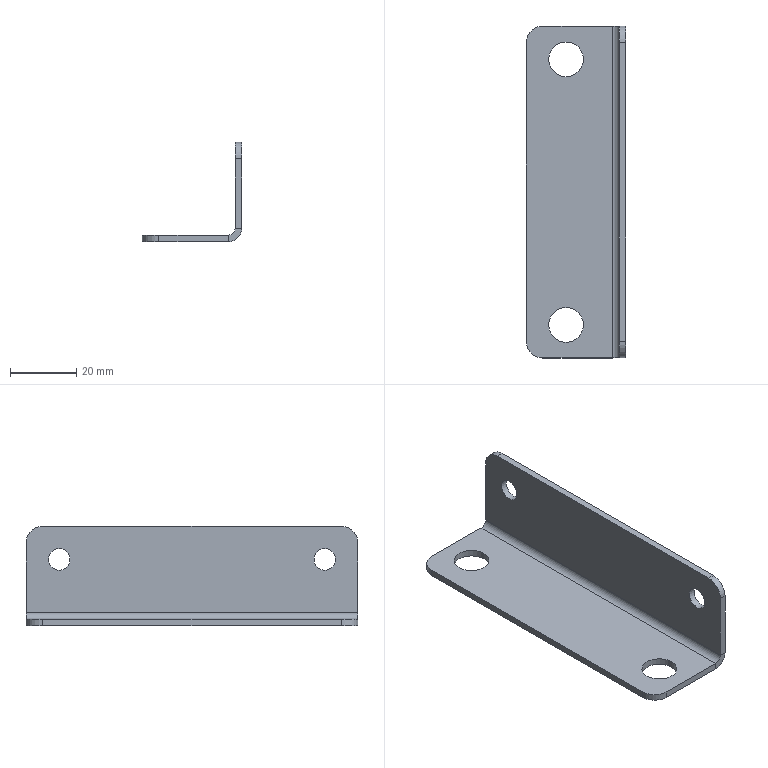Part | STEP file | JBJ-P-1006-07 | 1 solid | 22 faces | box 30 x 100 x 30 mm | volume 10820 mm3 | plane 12 | cylinder 10 | commonest cylinder face diameters 10 x4 6.5 x2 10.5 x2 4 x1 8 x1
STEP:
#1=CARTESIAN_POINT('',(30.,100.,4.));
#2=VERTEX_POINT('',#1);
#3=CARTESIAN_POINT('',(28.,100.,4.));
#4=VERTEX_POINT('',#3);
#5=CARTESIAN_POINT('',(30.,100.,4.));
#6=DIRECTION('',(-1.,0.,0.));
#7=VECTOR('',#6,1000.);
#8=LINE('',#5,#7);
#9=EDGE_CURVE('',#2,#4,#8,.T.);
#10=ORIENTED_EDGE('',*,*,#9,.F.);
#11=CARTESIAN_POINT('',(26.,100.,0.));
#12=VERTEX_POINT('',#11);
#13=CARTESIAN_POINT('',(26.,100.,4.));
#14=DIRECTION('',(0.,-1.,0.));
#15=DIRECTION('',(0.,0.,1.));
#16=AXIS2_PLACEMENT_3D('',#13,#14,#15);
#17=CIRCLE('',#16,4.);
#18=EDGE_CURVE('',#12,#2,#17,.T.);
#19=ORIENTED_EDGE('',*,*,#18,.F.);
#20=CARTESIAN_POINT('',(26.,100.,2.));
#21=VERTEX_POINT('',#20);
#22=CARTESIAN_POINT('',(26.,100.,2.));
#23=DIRECTION('',(0.,0.,-1.));
#24=VECTOR('',#23,1000.);
#25=LINE('',#22,#24);
#26=EDGE_CURVE('',#21,#12,#25,.T.);
#27=ORIENTED_EDGE('',*,*,#26,.F.);
#28=CARTESIAN_POINT('',(26.,100.,4.));
#29=DIRECTION('',(0.,-1.,0.));
#30=DIRECTION('',(1.,0.,0.));
#31=AXIS2_PLACEMENT_3D('',#28,#29,#30);
#32=CIRCLE('',#31,2.);
#33=EDGE_CURVE('',#21,#4,#32,.T.);
#34=ORIENTED_EDGE('',*,*,#33,.T.);
#35=EDGE_LOOP('',(#10,#19,#27,#34));
#36=FACE_OUTER_BOUND('',#35,.T.);
#37=CARTESIAN_POINT('',(30.,100.,4.));
#38=DIRECTION('',(0.,1.,0.));
#39=DIRECTION('',(0.,0.,1.));
#40=AXIS2_PLACEMENT_3D('',#37,#38,#39);
#41=PLANE('',#40);
#42=ADVANCED_FACE('',(#36),#41,.T.);
#43=CARTESIAN_POINT('',(28.,100.,25.));
#44=VERTEX_POINT('',#43);
#45=CARTESIAN_POINT('',(28.,100.,0.));
#46=DIRECTION('',(0.,0.,1.));
#47=VECTOR('',#46,1000.);
#48=LINE('',#45,#47);
#49=EDGE_CURVE('',#4,#44,#48,.T.);
#50=ORIENTED_EDGE('',*,*,#49,.T.);
#51=CARTESIAN_POINT('',(30.,100.,25.));
#52=VERTEX_POINT('',#51);
#53=CARTESIAN_POINT('',(26.,100.,25.));
#54=DIRECTION('',(1.,0.,0.));
#55=VECTOR('',#54,1000.);
#56=LINE('',#53,#55);
#57=EDGE_CURVE('',#44,#52,#56,.T.);
#58=ORIENTED_EDGE('',*,*,#57,.T.);
#59=CARTESIAN_POINT('',(30.,100.,0.));
#60=DIRECTION('',(0.,0.,1.));
#61=VECTOR('',#60,1000.);
#62=LINE('',#59,#61);
#63=EDGE_CURVE('',#2,#52,#62,.T.);
#64=ORIENTED_EDGE('',*,*,#63,.F.);
#65=ORIENTED_EDGE('',*,*,#9,.T.);
#66=EDGE_LOOP('',(#50,#58,#64,#65));
#67=FACE_OUTER_BOUND('',#66,.T.);
#68=CARTESIAN_POINT('',(26.,100.,2.));
#69=DIRECTION('',(0.,1.,0.));
#70=DIRECTION('',(0.,0.,1.));
#71=AXIS2_PLACEMENT_3D('',#68,#69,#70);
#72=PLANE('',#71);
#73=ADVANCED_FACE('',(#67),#72,.T.);
#74=CARTESIAN_POINT('',(26.,0.,0.));
#75=VERTEX_POINT('',#74);
#76=CARTESIAN_POINT('',(26.,0.,2.));
#77=VERTEX_POINT('',#76);
#78=CARTESIAN_POINT('',(26.,0.,0.));
#79=DIRECTION('',(0.,0.,1.));
#80=VECTOR('',#79,1000.);
#81=LINE('',#78,#80);
#82=EDGE_CURVE('',#75,#77,#81,.T.);
#83=ORIENTED_EDGE('',*,*,#82,.F.);
#84=CARTESIAN_POINT('',(30.,0.,4.));
#85=VERTEX_POINT('',#84);
#86=CARTESIAN_POINT('',(26.,0.,4.));
#87=DIRECTION('',(0.,-1.,0.));
#88=DIRECTION('',(0.,0.,1.));
#89=AXIS2_PLACEMENT_3D('',#86,#87,#88);
#90=CIRCLE('',#89,4.);
#91=EDGE_CURVE('',#75,#85,#90,.T.);
#92=ORIENTED_EDGE('',*,*,#91,.T.);
#93=CARTESIAN_POINT('',(28.,0.,4.));
#94=VERTEX_POINT('',#93);
#95=CARTESIAN_POINT('',(28.,0.,4.));
#96=DIRECTION('',(1.,0.,0.));
#97=VECTOR('',#96,1000.);
#98=LINE('',#95,#97);
#99=EDGE_CURVE('',#94,#85,#98,.T.);
#100=ORIENTED_EDGE('',*,*,#99,.F.);
#101=CARTESIAN_POINT('',(26.,0.,4.));
#102=DIRECTION('',(0.,-1.,0.));
#103=DIRECTION('',(1.,0.,0.));
#104=AXIS2_PLACEMENT_3D('',#101,#102,#103);
#105=CIRCLE('',#104,2.);
#106=EDGE_CURVE('',#77,#94,#105,.T.);
#107=ORIENTED_EDGE('',*,*,#106,.F.);
#108=EDGE_LOOP('',(#83,#92,#100,#107));
#109=FACE_OUTER_BOUND('',#108,.T.);
#110=CARTESIAN_POINT('',(26.,0.,0.));
#111=DIRECTION('',(0.,-1.,0.));
#112=DIRECTION('',(0.,0.,-1.));
#113=AXIS2_PLACEMENT_3D('',#110,#111,#112);
#114=PLANE('',#113);
#115=ADVANCED_FACE('',(#109),#114,.T.);
#116=CARTESIAN_POINT('',(5.,0.,2.));
#117=VERTEX_POINT('',#116);
#118=CARTESIAN_POINT('',(0.,0.,2.));
#119=DIRECTION('',(1.,0.,0.));
#120=VECTOR('',#119,1000.);
#121=LINE('',#118,#120);
#122=EDGE_CURVE('',#117,#77,#121,.T.);
#123=ORIENTED_EDGE('',*,*,#122,.F.);
#124=CARTESIAN_POINT('',(5.,0.,0.));
#125=VERTEX_POINT('',#124);
#126=CARTESIAN_POINT('',(5.,0.,4.));
#127=DIRECTION('',(0.,0.,-1.));
#128=VECTOR('',#127,1000.);
#129=LINE('',#126,#128);
#130=EDGE_CURVE('',#117,#125,#129,.T.);
#131=ORIENTED_EDGE('',*,*,#130,.T.);
#132=CARTESIAN_POINT('',(0.,0.,0.));
#133=DIRECTION('',(1.,0.,0.));
#134=VECTOR('',#133,1000.);
#135=LINE('',#132,#134);
#136=EDGE_CURVE('',#125,#75,#135,.T.);
#137=ORIENTED_EDGE('',*,*,#136,.T.);
#138=ORIENTED_EDGE('',*,*,#82,.T.);
#139=EDGE_LOOP('',(#123,#131,#137,#138));
#140=FACE_OUTER_BOUND('',#139,.T.);
#141=CARTESIAN_POINT('',(28.,0.,4.));
#142=DIRECTION('',(0.,-1.,0.));
#143=DIRECTION('',(0.,0.,-1.));
#144=AXIS2_PLACEMENT_3D('',#141,#142,#143);
#145=PLANE('',#144);
#146=ADVANCED_FACE('',(#140),#145,.T.);
#147=CARTESIAN_POINT('',(28.,90.,16.75));
#148=VERTEX_POINT('',#147);
#149=CARTESIAN_POINT('',(28.,90.,20.));
#150=DIRECTION('',(1.,0.,0.));
#151=DIRECTION('',(0.,0.,-1.));
#152=AXIS2_PLACEMENT_3D('',#149,#150,#151);
#153=CIRCLE('',#152,3.25);
#154=EDGE_CURVE('',#148,#148,#153,.T.);
#155=ORIENTED_EDGE('',*,*,#154,.T.);
#156=EDGE_LOOP('',(#155));
#157=FACE_BOUND('',#156,.T.);
#158=CARTESIAN_POINT('',(28.,10.,16.75));
#159=VERTEX_POINT('',#158);
#160=CARTESIAN_POINT('',(28.,10.,20.));
#161=DIRECTION('',(1.,0.,0.));
#162=DIRECTION('',(0.,0.,-1.));
#163=AXIS2_PLACEMENT_3D('',#160,#161,#162);
#164=CIRCLE('',#163,3.25);
#165=EDGE_CURVE('',#159,#159,#164,.T.);
#166=ORIENTED_EDGE('',*,*,#165,.T.);
#167=EDGE_LOOP('',(#166));
#168=FACE_BOUND('',#167,.T.);
#169=CARTESIAN_POINT('',(28.,95.,30.));
#170=VERTEX_POINT('',#169);
#171=CARTESIAN_POINT('',(28.,5.,30.));
#172=VERTEX_POINT('',#171);
#173=CARTESIAN_POINT('',(28.,100.,30.));
#174=DIRECTION('',(0.,-1.,0.));
#175=VECTOR('',#174,1000.);
#176=LINE('',#173,#175);
#177=EDGE_CURVE('',#170,#172,#176,.T.);
#178=ORIENTED_EDGE('',*,*,#177,.F.);
#179=CARTESIAN_POINT('',(28.,95.,25.));
#180=DIRECTION('',(-1.,0.,0.));
#181=DIRECTION('',(0.,0.,-1.));
#182=AXIS2_PLACEMENT_3D('',#179,#180,#181);
#183=CIRCLE('',#182,5.);
#184=EDGE_CURVE('',#170,#44,#183,.T.);
#185=ORIENTED_EDGE('',*,*,#184,.T.);
#186=ORIENTED_EDGE('',*,*,#49,.F.);
#187=CARTESIAN_POINT('',(28.,100.,4.));
#188=DIRECTION('',(0.,-1.,0.));
#189=VECTOR('',#188,1000.);
#190=LINE('',#187,#189);
#191=EDGE_CURVE('',#4,#94,#190,.T.);
#192=ORIENTED_EDGE('',*,*,#191,.T.);
#193=CARTESIAN_POINT('',(28.,0.,25.));
#194=VERTEX_POINT('',#193);
#195=CARTESIAN_POINT('',(28.,0.,0.));
#196=DIRECTION('',(0.,0.,1.));
#197=VECTOR('',#196,1000.);
#198=LINE('',#195,#197);
#199=EDGE_CURVE('',#94,#194,#198,.T.);
#200=ORIENTED_EDGE('',*,*,#199,.T.);
#201=CARTESIAN_POINT('',(28.,5.,25.));
#202=DIRECTION('',(-1.,0.,0.));
#203=DIRECTION('',(0.,0.,-1.));
#204=AXIS2_PLACEMENT_3D('',#201,#202,#203);
#205=CIRCLE('',#204,5.);
#206=EDGE_CURVE('',#194,#172,#205,.T.);
#207=ORIENTED_EDGE('',*,*,#206,.T.);
#208=EDGE_LOOP('',(#178,#185,#186,#192,#200,#207));
#209=FACE_OUTER_BOUND('',#208,.T.);
#210=CARTESIAN_POINT('',(28.,100.,0.));
#211=DIRECTION('',(1.,0.,0.));
#212=DIRECTION('',(0.,0.,-1.));
#213=AXIS2_PLACEMENT_3D('',#210,#211,#212);
#214=PLANE('',#213);
#215=ADVANCED_FACE('',(#157,#168,#209),#214,.F.);
#216=CARTESIAN_POINT('',(30.,95.,30.));
#217=VERTEX_POINT('',#216);
#218=CARTESIAN_POINT('',(30.,5.,30.));
#219=VERTEX_POINT('',#218);
#220=CARTESIAN_POINT('',(30.,100.,30.));
#221=DIRECTION('',(0.,-1.,0.));
#222=VECTOR('',#221,1000.);
#223=LINE('',#220,#222);
#224=EDGE_CURVE('',#217,#219,#223,.T.);
#225=ORIENTED_EDGE('',*,*,#224,.F.);
#226=CARTESIAN_POINT('',(30.,95.,30.));
#227=DIRECTION('',(-1.,0.,0.));
#228=VECTOR('',#227,1000.);
#229=LINE('',#226,#228);
#230=EDGE_CURVE('',#217,#170,#229,.T.);
#231=ORIENTED_EDGE('',*,*,#230,.T.);
#232=ORIENTED_EDGE('',*,*,#177,.T.);
#233=CARTESIAN_POINT('',(30.,5.,30.));
#234=DIRECTION('',(1.,0.,0.));
#235=VECTOR('',#234,1000.);
#236=LINE('',#233,#235);
#237=EDGE_CURVE('',#172,#219,#236,.T.);
#238=ORIENTED_EDGE('',*,*,#237,.T.);
#239=EDGE_LOOP('',(#225,#231,#232,#238));
#240=FACE_OUTER_BOUND('',#239,.T.);
#241=CARTESIAN_POINT('',(30.,100.,30.));
#242=DIRECTION('',(0.,0.,1.));
#243=DIRECTION('',(1.,0.,0.));
#244=AXIS2_PLACEMENT_3D('',#241,#242,#243);
#245=PLANE('',#244);
#246=ADVANCED_FACE('',(#240),#245,.T.);
#247=CARTESIAN_POINT('',(30.,90.,16.75));
#248=VERTEX_POINT('',#247);
#249=CARTESIAN_POINT('',(30.,90.,20.));
#250=DIRECTION('',(1.,0.,0.));
#251=DIRECTION('',(0.,0.,-1.));
#252=AXIS2_PLACEMENT_3D('',#249,#250,#251);
#253=CIRCLE('',#252,3.25);
#254=EDGE_CURVE('',#248,#248,#253,.T.);
#255=ORIENTED_EDGE('',*,*,#254,.F.);
#256=EDGE_LOOP('',(#255));
#257=FACE_BOUND('',#256,.T.);
#258=CARTESIAN_POINT('',(30.,10.,16.75));
#259=VERTEX_POINT('',#258);
#260=CARTESIAN_POINT('',(30.,10.,20.));
#261=DIRECTION('',(1.,0.,0.));
#262=DIRECTION('',(0.,0.,-1.));
#263=AXIS2_PLACEMENT_3D('',#260,#261,#262);
#264=CIRCLE('',#263,3.25);
#265=EDGE_CURVE('',#259,#259,#264,.T.);
#266=ORIENTED_EDGE('',*,*,#265,.F.);
#267=EDGE_LOOP('',(#266));
#268=FACE_BOUND('',#267,.T.);
#269=ORIENTED_EDGE('',*,*,#63,.T.);
#270=CARTESIAN_POINT('',(30.,95.,25.));
#271=DIRECTION('',(1.,0.,0.));
#272=DIRECTION('',(0.,0.,-1.));
#273=AXIS2_PLACEMENT_3D('',#270,#271,#272);
#274=CIRCLE('',#273,5.);
#275=EDGE_CURVE('',#52,#217,#274,.T.);
#276=ORIENTED_EDGE('',*,*,#275,.T.);
#277=ORIENTED_EDGE('',*,*,#224,.T.);
#278=CARTESIAN_POINT('',(30.,0.,25.));
#279=VERTEX_POINT('',#278);
#280=CARTESIAN_POINT('',(30.,5.,25.));
#281=DIRECTION('',(1.,0.,0.));
#282=DIRECTION('',(0.,0.,-1.));
#283=AXIS2_PLACEMENT_3D('',#280,#281,#282);
#284=CIRCLE('',#283,5.);
#285=EDGE_CURVE('',#219,#279,#284,.T.);
#286=ORIENTED_EDGE('',*,*,#285,.T.);
#287=CARTESIAN_POINT('',(30.,0.,0.));
#288=DIRECTION('',(0.,0.,1.));
#289=VECTOR('',#288,1000.);
#290=LINE('',#287,#289);
#291=EDGE_CURVE('',#85,#279,#290,.T.);
#292=ORIENTED_EDGE('',*,*,#291,.F.);
#293=CARTESIAN_POINT('',(30.,100.,4.));
#294=DIRECTION('',(0.,-1.,0.));
#295=VECTOR('',#294,1000.);
#296=LINE('',#293,#295);
#297=EDGE_CURVE('',#2,#85,#296,.T.);
#298=ORIENTED_EDGE('',*,*,#297,.F.);
#299=EDGE_LOOP('',(#269,#276,#277,#286,#292,#298));
#300=FACE_OUTER_BOUND('',#299,.T.);
#301=CARTESIAN_POINT('',(30.,100.,0.));
#302=DIRECTION('',(1.,0.,0.));
#303=DIRECTION('',(0.,0.,-1.));
#304=AXIS2_PLACEMENT_3D('',#301,#302,#303);
#305=PLANE('',#304);
#306=ADVANCED_FACE('',(#257,#268,#300),#305,.T.);
#307=ORIENTED_EDGE('',*,*,#91,.F.);
#308=CARTESIAN_POINT('',(26.,100.,0.));
#309=DIRECTION('',(0.,-1.,0.));
#310=VECTOR('',#309,1000.);
#311=LINE('',#308,#310);
#312=EDGE_CURVE('',#12,#75,#311,.T.);
#313=ORIENTED_EDGE('',*,*,#312,.F.);
#314=ORIENTED_EDGE('',*,*,#18,.T.);
#315=ORIENTED_EDGE('',*,*,#297,.T.);
#316=EDGE_LOOP('',(#307,#313,#314,#315));
#317=FACE_OUTER_BOUND('',#316,.T.);
#318=CARTESIAN_POINT('',(26.,100.,4.));
#319=DIRECTION('',(0.,-1.,0.));
#320=DIRECTION('',(0.,0.,-1.));
#321=AXIS2_PLACEMENT_3D('',#318,#319,#320);
#322=CYLINDRICAL_SURFACE('',#321,4.);
#323=ADVANCED_FACE('',(#317),#322,.T.);
#324=CARTESIAN_POINT('',(6.75,90.,0.));
#325=VERTEX_POINT('',#324);
#326=CARTESIAN_POINT('',(12.,90.,0.));
#327=DIRECTION('',(0.,0.,-1.));
#328=DIRECTION('',(-1.,0.,0.));
#329=AXIS2_PLACEMENT_3D('',#326,#327,#328);
#330=CIRCLE('',#329,5.25);
#331=EDGE_CURVE('',#325,#325,#330,.T.);
#332=ORIENTED_EDGE('',*,*,#331,.F.);
#333=EDGE_LOOP('',(#332));
#334=FACE_BOUND('',#333,.T.);
#335=CARTESIAN_POINT('',(6.75,10.,0.));
#336=VERTEX_POINT('',#335);
#337=CARTESIAN_POINT('',(12.,10.,0.));
#338=DIRECTION('',(0.,0.,-1.));
#339=DIRECTION('',(-1.,0.,0.));
#340=AXIS2_PLACEMENT_3D('',#337,#338,#339);
#341=CIRCLE('',#340,5.25);
#342=EDGE_CURVE('',#336,#336,#341,.T.);
#343=ORIENTED_EDGE('',*,*,#342,.F.);
#344=EDGE_LOOP('',(#343));
#345=FACE_BOUND('',#344,.T.);
#346=CARTESIAN_POINT('',(0.,95.,0.));
#347=VERTEX_POINT('',#346);
#348=CARTESIAN_POINT('',(0.,5.,0.));
#349=VERTEX_POINT('',#348);
#350=CARTESIAN_POINT('',(0.,100.,0.));
#351=DIRECTION('',(0.,-1.,0.));
#352=VECTOR('',#351,1000.);
#353=LINE('',#350,#352);
#354=EDGE_CURVE('',#347,#349,#353,.T.);
#355=ORIENTED_EDGE('',*,*,#354,.F.);
#356=CARTESIAN_POINT('',(5.,100.,0.));
#357=VERTEX_POINT('',#356);
#358=CARTESIAN_POINT('',(5.,95.,0.));
#359=DIRECTION('',(0.,0.,-1.));
#360=DIRECTION('',(-1.,0.,0.));
#361=AXIS2_PLACEMENT_3D('',#358,#359,#360);
#362=CIRCLE('',#361,5.);
#363=EDGE_CURVE('',#347,#357,#362,.T.);
#364=ORIENTED_EDGE('',*,*,#363,.T.);
#365=CARTESIAN_POINT('',(0.,100.,0.));
#366=DIRECTION('',(1.,0.,0.));
#367=VECTOR('',#366,1000.);
#368=LINE('',#365,#367);
#369=EDGE_CURVE('',#357,#12,#368,.T.);
#370=ORIENTED_EDGE('',*,*,#369,.T.);
#371=ORIENTED_EDGE('',*,*,#312,.T.);
#372=ORIENTED_EDGE('',*,*,#136,.F.);
#373=CARTESIAN_POINT('',(5.,5.,0.));
#374=DIRECTION('',(0.,0.,-1.));
#375=DIRECTION('',(-1.,0.,0.));
#376=AXIS2_PLACEMENT_3D('',#373,#374,#375);
#377=CIRCLE('',#376,5.);
#378=EDGE_CURVE('',#125,#349,#377,.T.);
#379=ORIENTED_EDGE('',*,*,#378,.T.);
#380=EDGE_LOOP('',(#355,#364,#370,#371,#372,#379));
#381=FACE_OUTER_BOUND('',#380,.T.);
#382=CARTESIAN_POINT('',(0.,100.,0.));
#383=DIRECTION('',(0.,0.,-1.));
#384=DIRECTION('',(-1.,0.,0.));
#385=AXIS2_PLACEMENT_3D('',#382,#383,#384);
#386=PLANE('',#385);
#387=ADVANCED_FACE('',(#334,#345,#381),#386,.T.);
#388=CARTESIAN_POINT('',(0.,95.,2.));
#389=VERTEX_POINT('',#388);
#390=CARTESIAN_POINT('',(0.,5.,2.));
#391=VERTEX_POINT('',#390);
#392=CARTESIAN_POINT('',(0.,100.,2.));
#393=DIRECTION('',(0.,-1.,0.));
#394=VECTOR('',#393,1000.);
#395=LINE('',#392,#394);
#396=EDGE_CURVE('',#389,#391,#395,.T.);
#397=ORIENTED_EDGE('',*,*,#396,.F.);
#398=CARTESIAN_POINT('',(0.,95.,2.));
#399=DIRECTION('',(0.,0.,-1.));
#400=VECTOR('',#399,1000.);
#401=LINE('',#398,#400);
#402=EDGE_CURVE('',#389,#347,#401,.T.);
#403=ORIENTED_EDGE('',*,*,#402,.T.);
#404=ORIENTED_EDGE('',*,*,#354,.T.);
#405=CARTESIAN_POINT('',(0.,5.,2.));
#406=DIRECTION('',(0.,0.,1.));
#407=VECTOR('',#406,1000.);
#408=LINE('',#405,#407);
#409=EDGE_CURVE('',#349,#391,#408,.T.);
#410=ORIENTED_EDGE('',*,*,#409,.T.);
#411=EDGE_LOOP('',(#397,#403,#404,#410));
#412=FACE_OUTER_BOUND('',#411,.T.);
#413=CARTESIAN_POINT('',(0.,100.,2.));
#414=DIRECTION('',(-1.,0.,0.));
#415=DIRECTION('',(0.,0.,1.));
#416=AXIS2_PLACEMENT_3D('',#413,#414,#415);
#417=PLANE('',#416);
#418=ADVANCED_FACE('',(#412),#417,.T.);
#419=CARTESIAN_POINT('',(17.25,90.,2.));
#420=VERTEX_POINT('',#419);
#421=CARTESIAN_POINT('',(12.,90.,2.));
#422=DIRECTION('',(0.,0.,1.));
#423=DIRECTION('',(1.,0.,0.));
#424=AXIS2_PLACEMENT_3D('',#421,#422,#423);
#425=CIRCLE('',#424,5.25);
#426=EDGE_CURVE('',#420,#420,#425,.T.);
#427=ORIENTED_EDGE('',*,*,#426,.F.);
#428=EDGE_LOOP('',(#427));
#429=FACE_BOUND('',#428,.T.);
#430=CARTESIAN_POINT('',(17.25,10.,2.));
#431=VERTEX_POINT('',#430);
#432=CARTESIAN_POINT('',(12.,10.,2.));
#433=DIRECTION('',(0.,0.,1.));
#434=DIRECTION('',(1.,0.,0.));
#435=AXIS2_PLACEMENT_3D('',#432,#433,#434);
#436=CIRCLE('',#435,5.25);
#437=EDGE_CURVE('',#431,#431,#436,.T.);
#438=ORIENTED_EDGE('',*,*,#437,.F.);
#439=EDGE_LOOP('',(#438));
#440=FACE_BOUND('',#439,.T.);
#441=CARTESIAN_POINT('',(5.,100.,2.));
#442=VERTEX_POINT('',#441);
#443=CARTESIAN_POINT('',(0.,100.,2.));
#444=DIRECTION('',(1.,0.,0.));
#445=VECTOR('',#444,1000.);
#446=LINE('',#443,#445);
#447=EDGE_CURVE('',#442,#21,#446,.T.);
#448=ORIENTED_EDGE('',*,*,#447,.F.);
#449=CARTESIAN_POINT('',(5.,95.,2.));
#450=DIRECTION('',(0.,0.,1.));
#451=DIRECTION('',(-1.,0.,0.));
#452=AXIS2_PLACEMENT_3D('',#449,#450,#451);
#453=CIRCLE('',#452,5.);
#454=EDGE_CURVE('',#442,#389,#453,.T.);
#455=ORIENTED_EDGE('',*,*,#454,.T.);
#456=ORIENTED_EDGE('',*,*,#396,.T.);
#457=CARTESIAN_POINT('',(5.,5.,2.));
#458=DIRECTION('',(0.,0.,1.));
#459=DIRECTION('',(-1.,0.,0.));
#460=AXIS2_PLACEMENT_3D('',#457,#458,#459);
#461=CIRCLE('',#460,5.);
#462=EDGE_CURVE('',#391,#117,#461,.T.);
#463=ORIENTED_EDGE('',*,*,#462,.T.);
#464=ORIENTED_EDGE('',*,*,#122,.T.);
#465=CARTESIAN_POINT('',(26.,100.,2.));
#466=DIRECTION('',(0.,-1.,0.));
#467=VECTOR('',#466,1000.);
#468=LINE('',#465,#467);
#469=EDGE_CURVE('',#21,#77,#468,.T.);
#470=ORIENTED_EDGE('',*,*,#469,.F.);
#471=EDGE_LOOP('',(#448,#455,#456,#463,#464,#470));
#472=FACE_OUTER_BOUND('',#471,.T.);
#473=CARTESIAN_POINT('',(0.,100.,2.));
#474=DIRECTION('',(0.,0.,-1.));
#475=DIRECTION('',(-1.,0.,0.));
#476=AXIS2_PLACEMENT_3D('',#473,#474,#475);
#477=PLANE('',#476);
#478=ADVANCED_FACE('',(#429,#440,#472),#477,.F.);
#479=ORIENTED_EDGE('',*,*,#106,.T.);
#480=ORIENTED_EDGE('',*,*,#191,.F.);
#481=ORIENTED_EDGE('',*,*,#33,.F.);
#482=ORIENTED_EDGE('',*,*,#469,.T.);
#483=EDGE_LOOP('',(#479,#480,#481,#482));
#484=FACE_OUTER_BOUND('',#483,.T.);
#485=CARTESIAN_POINT('',(26.,100.,4.));
#486=DIRECTION('',(0.,-1.,0.));
#487=DIRECTION('',(0.,0.,-1.));
#488=AXIS2_PLACEMENT_3D('',#485,#486,#487);
#489=CYLINDRICAL_SURFACE('',#488,2.);
#490=ADVANCED_FACE('',(#484),#489,.F.);
#491=ORIENTED_EDGE('',*,*,#369,.F.);
#492=CARTESIAN_POINT('',(5.,100.,4.));
#493=DIRECTION('',(0.,0.,1.));
#494=VECTOR('',#493,1000.);
#495=LINE('',#492,#494);
#496=EDGE_CURVE('',#357,#442,#495,.T.);
#497=ORIENTED_EDGE('',*,*,#496,.T.);
#498=ORIENTED_EDGE('',*,*,#447,.T.);
#499=ORIENTED_EDGE('',*,*,#26,.T.);
#500=EDGE_LOOP('',(#491,#497,#498,#499));
#501=FACE_OUTER_BOUND('',#500,.T.);
#502=CARTESIAN_POINT('',(26.,100.,4.));
#503=DIRECTION('',(0.,1.,0.));
#504=DIRECTION('',(1.,0.,0.));
#505=AXIS2_PLACEMENT_3D('',#502,#503,#504);
#506=PLANE('',#505);
#507=ADVANCED_FACE('',(#501),#506,.T.);
#508=ORIENTED_EDGE('',*,*,#291,.T.);
#509=CARTESIAN_POINT('',(28.,0.,25.));
#510=DIRECTION('',(-1.,0.,0.));
#511=VECTOR('',#510,1000.);
#512=LINE('',#509,#511);
#513=EDGE_CURVE('',#279,#194,#512,.T.);
#514=ORIENTED_EDGE('',*,*,#513,.T.);
#515=ORIENTED_EDGE('',*,*,#199,.F.);
#516=ORIENTED_EDGE('',*,*,#99,.T.);
#517=EDGE_LOOP('',(#508,#514,#515,#516));
#518=FACE_OUTER_BOUND('',#517,.T.);
#519=CARTESIAN_POINT('',(26.,0.,4.));
#520=DIRECTION('',(0.,1.,0.));
#521=DIRECTION('',(1.,0.,0.));
#522=AXIS2_PLACEMENT_3D('',#519,#520,#521);
#523=PLANE('',#522);
#524=ADVANCED_FACE('',(#518),#523,.F.);
#525=ORIENTED_EDGE('',*,*,#275,.F.);
#526=ORIENTED_EDGE('',*,*,#57,.F.);
#527=ORIENTED_EDGE('',*,*,#184,.F.);
#528=ORIENTED_EDGE('',*,*,#230,.F.);
#529=EDGE_LOOP('',(#525,#526,#527,#528));
#530=FACE_OUTER_BOUND('',#529,.T.);
#531=CARTESIAN_POINT('',(30.,95.,25.));
#532=DIRECTION('',(-1.,0.,0.));
#533=DIRECTION('',(0.,0.,1.));
#534=AXIS2_PLACEMENT_3D('',#531,#532,#533);
#535=CYLINDRICAL_SURFACE('',#534,5.);
#536=ADVANCED_FACE('',(#530),#535,.T.);
#537=ORIENTED_EDGE('',*,*,#454,.F.);
#538=ORIENTED_EDGE('',*,*,#496,.F.);
#539=ORIENTED_EDGE('',*,*,#363,.F.);
#540=ORIENTED_EDGE('',*,*,#402,.F.);
#541=EDGE_LOOP('',(#537,#538,#539,#540));
#542=FACE_OUTER_BOUND('',#541,.T.);
#543=CARTESIAN_POINT('',(5.,95.,2.));
#544=DIRECTION('',(0.,0.,-1.));
#545=DIRECTION('',(-1.,0.,0.));
#546=AXIS2_PLACEMENT_3D('',#543,#544,#545);
#547=CYLINDRICAL_SURFACE('',#546,5.);
#548=ADVANCED_FACE('',(#542),#547,.T.);
#549=ORIENTED_EDGE('',*,*,#462,.F.);
#550=ORIENTED_EDGE('',*,*,#409,.F.);
#551=ORIENTED_EDGE('',*,*,#378,.F.);
#552=ORIENTED_EDGE('',*,*,#130,.F.);
#553=EDGE_LOOP('',(#549,#550,#551,#552));
#554=FACE_OUTER_BOUND('',#553,.T.);
#555=CARTESIAN_POINT('',(5.,5.,4.));
#556=DIRECTION('',(0.,0.,-1.));
#557=DIRECTION('',(-1.,0.,0.));
#558=AXIS2_PLACEMENT_3D('',#555,#556,#557);
#559=CYLINDRICAL_SURFACE('',#558,5.);
#560=ADVANCED_FACE('',(#554),#559,.T.);
#561=ORIENTED_EDGE('',*,*,#285,.F.);
#562=ORIENTED_EDGE('',*,*,#237,.F.);
#563=ORIENTED_EDGE('',*,*,#206,.F.);
#564=ORIENTED_EDGE('',*,*,#513,.F.);
#565=EDGE_LOOP('',(#561,#562,#563,#564));
#566=FACE_OUTER_BOUND('',#565,.T.);
#567=CARTESIAN_POINT('',(26.,5.,25.));
#568=DIRECTION('',(1.,0.,0.));
#569=DIRECTION('',(0.,0.,-1.));
#570=AXIS2_PLACEMENT_3D('',#567,#568,#569);
#571=CYLINDRICAL_SURFACE('',#570,5.);
#572=ADVANCED_FACE('',(#566),#571,.T.);
#573=ORIENTED_EDGE('',*,*,#437,.T.);
#574=EDGE_LOOP('',(#573));
#575=FACE_OUTER_BOUND('',#574,.T.);
#576=ORIENTED_EDGE('',*,*,#342,.T.);
#577=EDGE_LOOP('',(#576));
#578=FACE_OUTER_BOUND('',#577,.T.);
#579=CARTESIAN_POINT('',(12.,10.,2.));
#580=DIRECTION('',(0.,0.,1.));
#581=DIRECTION('',(1.,0.,0.));
#582=AXIS2_PLACEMENT_3D('',#579,#580,#581);
#583=CYLINDRICAL_SURFACE('',#582,5.25);
#584=ADVANCED_FACE('',(#575,#578),#583,.F.);
#585=ORIENTED_EDGE('',*,*,#426,.T.);
#586=EDGE_LOOP('',(#585));
#587=FACE_OUTER_BOUND('',#586,.T.);
#588=ORIENTED_EDGE('',*,*,#331,.T.);
#589=EDGE_LOOP('',(#588));
#590=FACE_OUTER_BOUND('',#589,.T.);
#591=CARTESIAN_POINT('',(12.,90.,2.));
#592=DIRECTION('',(0.,0.,1.));
#593=DIRECTION('',(1.,0.,0.));
#594=AXIS2_PLACEMENT_3D('',#591,#592,#593);
#595=CYLINDRICAL_SURFACE('',#594,5.25);
#596=ADVANCED_FACE('',(#587,#590),#595,.F.);
#597=ORIENTED_EDGE('',*,*,#265,.T.);
#598=EDGE_LOOP('',(#597));
#599=FACE_OUTER_BOUND('',#598,.T.);
#600=ORIENTED_EDGE('',*,*,#165,.F.);
#601=EDGE_LOOP('',(#600));
#602=FACE_OUTER_BOUND('',#601,.T.);
#603=CARTESIAN_POINT('',(30.,10.,20.));
#604=DIRECTION('',(1.,0.,0.));
#605=DIRECTION('',(0.,0.,-1.));
#606=AXIS2_PLACEMENT_3D('',#603,#604,#605);
#607=CYLINDRICAL_SURFACE('',#606,3.25);
#608=ADVANCED_FACE('',(#599,#602),#607,.F.);
#609=ORIENTED_EDGE('',*,*,#254,.T.);
#610=EDGE_LOOP('',(#609));
#611=FACE_OUTER_BOUND('',#610,.T.);
#612=ORIENTED_EDGE('',*,*,#154,.F.);
#613=EDGE_LOOP('',(#612));
#614=FACE_OUTER_BOUND('',#613,.T.);
#615=CARTESIAN_POINT('',(30.,90.,20.));
#616=DIRECTION('',(1.,0.,0.));
#617=DIRECTION('',(0.,0.,-1.));
#618=AXIS2_PLACEMENT_3D('',#615,#616,#617);
#619=CYLINDRICAL_SURFACE('',#618,3.25);
#620=ADVANCED_FACE('',(#611,#614),#619,.F.);
#621=CLOSED_SHELL('',(#42,#73,#115,#146,#215,#246,#306,#323,#387,#418,#478,#490,#507,#524,#536,#548,#560,#572,#584,#596,#608,#620));
#622=MANIFOLD_SOLID_BREP('',#621);
#623=CARTESIAN_POINT('',(0.,0.,0.));
#624=DIRECTION('',(0.,0.,1.));
#625=DIRECTION('',(1.,0.,0.));
#626=AXIS2_PLACEMENT_3D('',#623,#624,#625);
#627=(LENGTH_UNIT()NAMED_UNIT(*)SI_UNIT(.MILLI.,.METRE.));
#628=UNCERTAINTY_MEASURE_WITH_UNIT(LENGTH_MEASURE(0.00001),#627,'','');
#629=(NAMED_UNIT(*)PLANE_ANGLE_UNIT()SI_UNIT($,.RADIAN.));
#630=(NAMED_UNIT(*)SI_UNIT($,.STERADIAN.)SOLID_ANGLE_UNIT());
#631=(GEOMETRIC_REPRESENTATION_CONTEXT(3)GLOBAL_UNCERTAINTY_ASSIGNED_CONTEXT((#628))GLOBAL_UNIT_ASSIGNED_CONTEXT((#627,#629,#630))REPRESENTATION_CONTEXT('',''));
#632=ADVANCED_BREP_SHAPE_REPRESENTATION('',(#622,#626),#631);